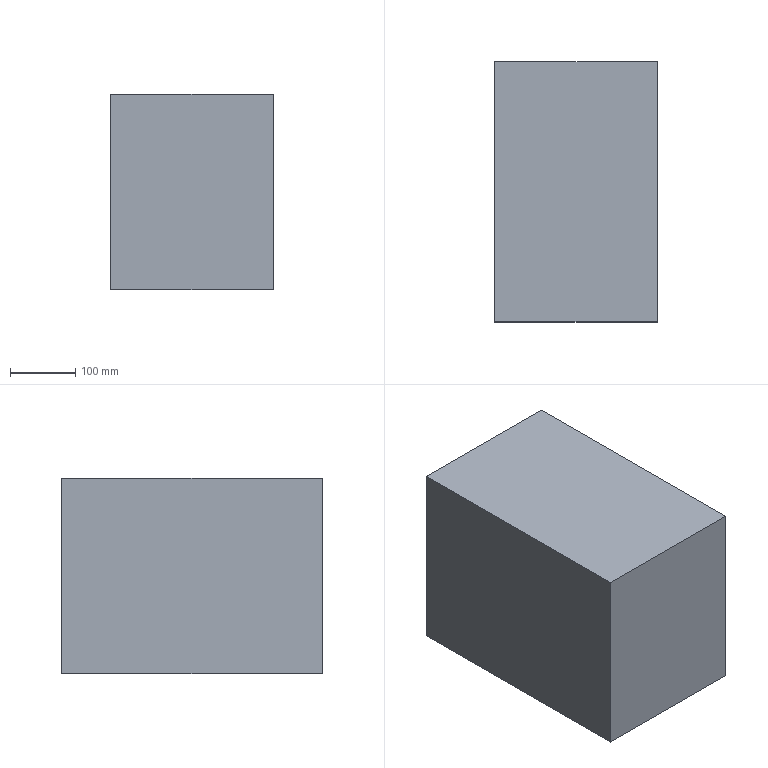Part | SolidWorks | features Extrusion 1 | 1 solid | 6 faces | box 250 x 400 x 300 mm | volume 30000000 mm3 | plane 6
STEP:
#1=CARTESIAN_POINT('',(125.,-200.,0.));
#2=VERTEX_POINT('',#1);
#3=CARTESIAN_POINT('',(125.,200.,0.));
#4=VERTEX_POINT('',#3);
#5=CARTESIAN_POINT('',(125.,200.,0.));
#6=DIRECTION('',(0.,1.,0.));
#7=VECTOR('',#6,1000.);
#8=LINE('',#5,#7);
#9=EDGE_CURVE('',#2,#4,#8,.T.);
#10=ORIENTED_EDGE('',*,*,#9,.T.);
#11=CARTESIAN_POINT('',(125.,200.,300.));
#12=VERTEX_POINT('',#11);
#13=CARTESIAN_POINT('',(125.,200.,300.));
#14=DIRECTION('',(0.,0.,-1.));
#15=VECTOR('',#14,1000.);
#16=LINE('',#13,#15);
#17=EDGE_CURVE('',#12,#4,#16,.T.);
#18=ORIENTED_EDGE('',*,*,#17,.F.);
#19=CARTESIAN_POINT('',(125.,-200.,300.));
#20=VERTEX_POINT('',#19);
#21=CARTESIAN_POINT('',(125.,200.,300.));
#22=DIRECTION('',(0.,1.,0.));
#23=VECTOR('',#22,1000.);
#24=LINE('',#21,#23);
#25=EDGE_CURVE('',#20,#12,#24,.T.);
#26=ORIENTED_EDGE('',*,*,#25,.F.);
#27=CARTESIAN_POINT('',(125.,-200.,300.));
#28=DIRECTION('',(0.,0.,-1.));
#29=VECTOR('',#28,1000.);
#30=LINE('',#27,#29);
#31=EDGE_CURVE('',#20,#2,#30,.T.);
#32=ORIENTED_EDGE('',*,*,#31,.T.);
#33=EDGE_LOOP('',(#10,#18,#26,#32));
#34=FACE_OUTER_BOUND('',#33,.T.);
#35=CARTESIAN_POINT('',(125.,200.,300.));
#36=DIRECTION('',(-1.,0.,0.));
#37=DIRECTION('',(0.,-1.,0.));
#38=AXIS2_PLACEMENT_3D('',#35,#36,#37);
#39=PLANE('',#38);
#40=ADVANCED_FACE('',(#34),#39,.F.);
#41=CARTESIAN_POINT('',(-125.,200.,0.));
#42=VERTEX_POINT('',#41);
#43=CARTESIAN_POINT('',(-125.,200.,0.));
#44=DIRECTION('',(-1.,0.,0.));
#45=VECTOR('',#44,1000.);
#46=LINE('',#43,#45);
#47=EDGE_CURVE('',#4,#42,#46,.T.);
#48=ORIENTED_EDGE('',*,*,#47,.T.);
#49=CARTESIAN_POINT('',(-125.,200.,300.));
#50=VERTEX_POINT('',#49);
#51=CARTESIAN_POINT('',(-125.,200.,300.));
#52=DIRECTION('',(0.,0.,-1.));
#53=VECTOR('',#52,1000.);
#54=LINE('',#51,#53);
#55=EDGE_CURVE('',#50,#42,#54,.T.);
#56=ORIENTED_EDGE('',*,*,#55,.F.);
#57=CARTESIAN_POINT('',(-125.,200.,300.));
#58=DIRECTION('',(-1.,0.,0.));
#59=VECTOR('',#58,1000.);
#60=LINE('',#57,#59);
#61=EDGE_CURVE('',#12,#50,#60,.T.);
#62=ORIENTED_EDGE('',*,*,#61,.F.);
#63=ORIENTED_EDGE('',*,*,#17,.T.);
#64=EDGE_LOOP('',(#48,#56,#62,#63));
#65=FACE_OUTER_BOUND('',#64,.T.);
#66=CARTESIAN_POINT('',(-125.,200.,300.));
#67=DIRECTION('',(0.,-1.,0.));
#68=DIRECTION('',(0.,0.,-1.));
#69=AXIS2_PLACEMENT_3D('',#66,#67,#68);
#70=PLANE('',#69);
#71=ADVANCED_FACE('',(#65),#70,.F.);
#72=CARTESIAN_POINT('',(-125.,-200.,0.));
#73=VERTEX_POINT('',#72);
#74=CARTESIAN_POINT('',(-125.,200.,0.));
#75=DIRECTION('',(0.,-1.,0.));
#76=VECTOR('',#75,1000.);
#77=LINE('',#74,#76);
#78=EDGE_CURVE('',#42,#73,#77,.T.);
#79=ORIENTED_EDGE('',*,*,#78,.T.);
#80=CARTESIAN_POINT('',(-125.,-200.,300.));
#81=VERTEX_POINT('',#80);
#82=CARTESIAN_POINT('',(-125.,-200.,300.));
#83=DIRECTION('',(0.,0.,-1.));
#84=VECTOR('',#83,1000.);
#85=LINE('',#82,#84);
#86=EDGE_CURVE('',#81,#73,#85,.T.);
#87=ORIENTED_EDGE('',*,*,#86,.F.);
#88=CARTESIAN_POINT('',(-125.,200.,300.));
#89=DIRECTION('',(0.,-1.,0.));
#90=VECTOR('',#89,1000.);
#91=LINE('',#88,#90);
#92=EDGE_CURVE('',#50,#81,#91,.T.);
#93=ORIENTED_EDGE('',*,*,#92,.F.);
#94=ORIENTED_EDGE('',*,*,#55,.T.);
#95=EDGE_LOOP('',(#79,#87,#93,#94));
#96=FACE_OUTER_BOUND('',#95,.T.);
#97=CARTESIAN_POINT('',(-125.,200.,300.));
#98=DIRECTION('',(1.,0.,0.));
#99=DIRECTION('',(0.,1.,0.));
#100=AXIS2_PLACEMENT_3D('',#97,#98,#99);
#101=PLANE('',#100);
#102=ADVANCED_FACE('',(#96),#101,.F.);
#103=CARTESIAN_POINT('',(-125.,-200.,0.));
#104=DIRECTION('',(1.,0.,0.));
#105=VECTOR('',#104,1000.);
#106=LINE('',#103,#105);
#107=EDGE_CURVE('',#73,#2,#106,.T.);
#108=ORIENTED_EDGE('',*,*,#107,.T.);
#109=ORIENTED_EDGE('',*,*,#31,.F.);
#110=CARTESIAN_POINT('',(-125.,-200.,300.));
#111=DIRECTION('',(1.,0.,0.));
#112=VECTOR('',#111,1000.);
#113=LINE('',#110,#112);
#114=EDGE_CURVE('',#81,#20,#113,.T.);
#115=ORIENTED_EDGE('',*,*,#114,.F.);
#116=ORIENTED_EDGE('',*,*,#86,.T.);
#117=EDGE_LOOP('',(#108,#109,#115,#116));
#118=FACE_OUTER_BOUND('',#117,.T.);
#119=CARTESIAN_POINT('',(-125.,-200.,300.));
#120=DIRECTION('',(0.,1.,0.));
#121=DIRECTION('',(0.,0.,1.));
#122=AXIS2_PLACEMENT_3D('',#119,#120,#121);
#123=PLANE('',#122);
#124=ADVANCED_FACE('',(#118),#123,.F.);
#125=ORIENTED_EDGE('',*,*,#25,.T.);
#126=ORIENTED_EDGE('',*,*,#61,.T.);
#127=ORIENTED_EDGE('',*,*,#92,.T.);
#128=ORIENTED_EDGE('',*,*,#114,.T.);
#129=EDGE_LOOP('',(#125,#126,#127,#128));
#130=FACE_OUTER_BOUND('',#129,.T.);
#131=CARTESIAN_POINT('',(0.,0.,300.));
#132=DIRECTION('',(0.,0.,1.));
#133=DIRECTION('',(1.,0.,0.));
#134=AXIS2_PLACEMENT_3D('',#131,#132,#133);
#135=PLANE('',#134);
#136=ADVANCED_FACE('',(#130),#135,.T.);
#137=ORIENTED_EDGE('',*,*,#9,.F.);
#138=ORIENTED_EDGE('',*,*,#107,.F.);
#139=ORIENTED_EDGE('',*,*,#78,.F.);
#140=ORIENTED_EDGE('',*,*,#47,.F.);
#141=EDGE_LOOP('',(#137,#138,#139,#140));
#142=FACE_OUTER_BOUND('',#141,.T.);
#143=CARTESIAN_POINT('',(0.,0.,0.));
#144=DIRECTION('',(0.,0.,1.));
#145=DIRECTION('',(1.,0.,0.));
#146=AXIS2_PLACEMENT_3D('',#143,#144,#145);
#147=PLANE('',#146);
#148=ADVANCED_FACE('',(#142),#147,.F.);
#149=CLOSED_SHELL('',(#40,#71,#102,#124,#136,#148));
#150=MANIFOLD_SOLID_BREP('',#149);
#151=CARTESIAN_POINT('',(0.,0.,0.));
#152=DIRECTION('',(0.,0.,1.));
#153=DIRECTION('',(1.,0.,0.));
#154=AXIS2_PLACEMENT_3D('',#151,#152,#153);
#155=(LENGTH_UNIT()NAMED_UNIT(*)SI_UNIT(.MILLI.,.METRE.));
#156=UNCERTAINTY_MEASURE_WITH_UNIT(LENGTH_MEASURE(0.00001),#155,'','');
#157=(NAMED_UNIT(*)PLANE_ANGLE_UNIT()SI_UNIT($,.RADIAN.));
#158=(NAMED_UNIT(*)SI_UNIT($,.STERADIAN.)SOLID_ANGLE_UNIT());
#159=(GEOMETRIC_REPRESENTATION_CONTEXT(3)GLOBAL_UNCERTAINTY_ASSIGNED_CONTEXT((#156))GLOBAL_UNIT_ASSIGNED_CONTEXT((#155,#157,#158))REPRESENTATION_CONTEXT('',''));
#160=ADVANCED_BREP_SHAPE_REPRESENTATION('',(#150,#154),#159);